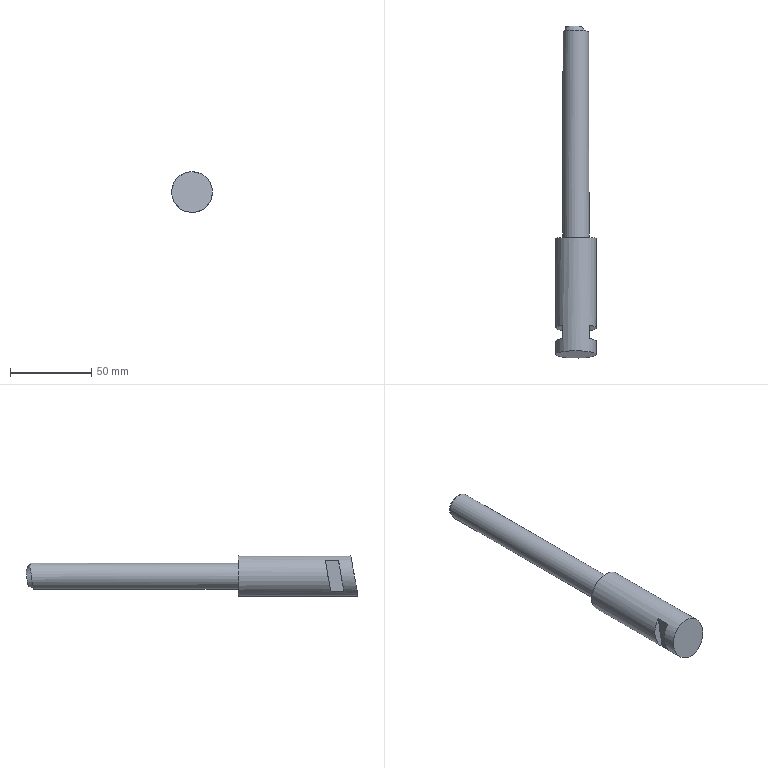Part | STEP file | solid 187 | 1 solid | 13 faces | box 25 x 204.048 x 25 mm | volume 59820 mm3 | plane 8 | spline 3 | cylinder 2 | commonest cylinder face diameters 16 x1 25 x1